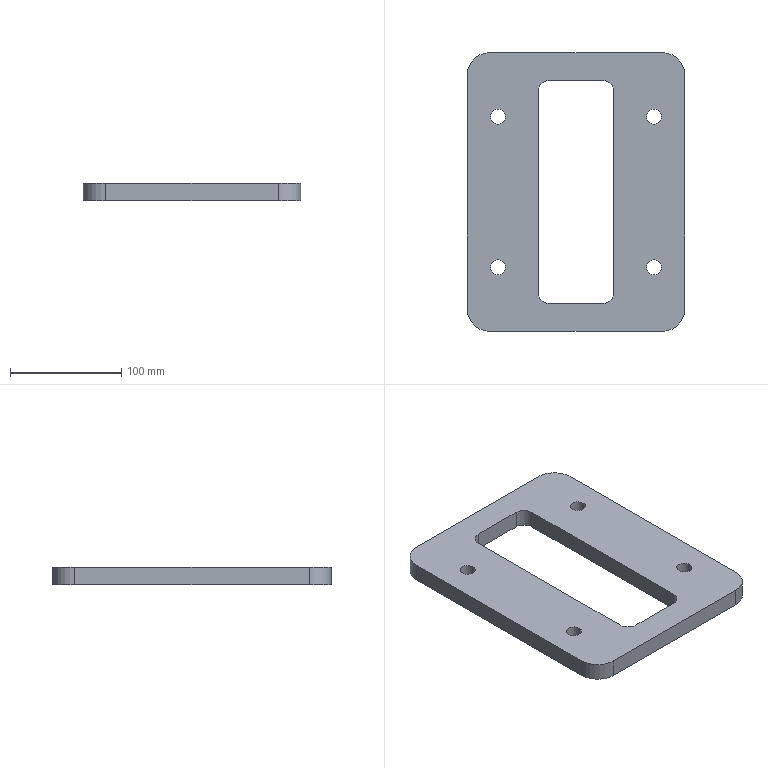Part | SolidWorks | features Fillet 2, Chamfer 1, Extrusion 1, HoleWzd 1 | 1 solid | 26 faces | box 195 x 250 x 16 mm | volume 549119 mm3 | cylinder 16 | plane 10 | commonest cylinder face diameters 13.5 x8 20 x4 40 x4
STEP:
#1=CARTESIAN_POINT('',(-76.75,67.5,-8.));
#2=VERTEX_POINT('',#1);
#3=CARTESIAN_POINT('',(-63.25,67.5,-8.));
#4=VERTEX_POINT('',#3);
#5=CARTESIAN_POINT('',(-70.,67.5,-8.));
#6=DIRECTION('',(0.,0.,1.));
#7=DIRECTION('',(1.,0.,0.));
#8=AXIS2_PLACEMENT_3D('',#5,#6,#7);
#9=CIRCLE('',#8,6.75);
#10=EDGE_CURVE('',#2,#4,#9,.T.);
#11=ORIENTED_EDGE('',*,*,#10,.F.);
#12=CARTESIAN_POINT('',(-76.75,67.5,8.));
#13=VERTEX_POINT('',#12);
#14=CARTESIAN_POINT('',(-76.75,67.5,8.));
#15=DIRECTION('',(0.,0.,1.));
#16=VECTOR('',#15,1000.);
#17=LINE('',#14,#16);
#18=EDGE_CURVE('',#2,#13,#17,.T.);
#19=ORIENTED_EDGE('',*,*,#18,.T.);
#20=CARTESIAN_POINT('',(-63.25,67.5,8.));
#21=VERTEX_POINT('',#20);
#22=CARTESIAN_POINT('',(-70.,67.5,8.));
#23=DIRECTION('',(0.,0.,1.));
#24=DIRECTION('',(1.,0.,0.));
#25=AXIS2_PLACEMENT_3D('',#22,#23,#24);
#26=CIRCLE('',#25,6.75);
#27=EDGE_CURVE('',#13,#21,#26,.T.);
#28=ORIENTED_EDGE('',*,*,#27,.T.);
#29=CARTESIAN_POINT('',(-63.25,67.5,8.));
#30=DIRECTION('',(0.,0.,1.));
#31=VECTOR('',#30,1000.);
#32=LINE('',#29,#31);
#33=EDGE_CURVE('',#4,#21,#32,.T.);
#34=ORIENTED_EDGE('',*,*,#33,.F.);
#35=EDGE_LOOP('',(#11,#19,#28,#34));
#36=FACE_OUTER_BOUND('',#35,.T.);
#37=CARTESIAN_POINT('',(-70.,67.5,8.));
#38=DIRECTION('',(0.,0.,1.));
#39=DIRECTION('',(1.,0.,0.));
#40=AXIS2_PLACEMENT_3D('',#37,#38,#39);
#41=CYLINDRICAL_SURFACE('',#40,6.75);
#42=ADVANCED_FACE('',(#36),#41,.F.);
#43=CARTESIAN_POINT('',(63.25,67.5,-8.));
#44=VERTEX_POINT('',#43);
#45=CARTESIAN_POINT('',(76.75,67.5,-8.));
#46=VERTEX_POINT('',#45);
#47=CARTESIAN_POINT('',(70.,67.5,-8.));
#48=DIRECTION('',(0.,0.,1.));
#49=DIRECTION('',(1.,0.,0.));
#50=AXIS2_PLACEMENT_3D('',#47,#48,#49);
#51=CIRCLE('',#50,6.75);
#52=EDGE_CURVE('',#44,#46,#51,.T.);
#53=ORIENTED_EDGE('',*,*,#52,.F.);
#54=CARTESIAN_POINT('',(63.25,67.5,8.));
#55=VERTEX_POINT('',#54);
#56=CARTESIAN_POINT('',(63.25,67.5,8.));
#57=DIRECTION('',(0.,0.,1.));
#58=VECTOR('',#57,1000.);
#59=LINE('',#56,#58);
#60=EDGE_CURVE('',#44,#55,#59,.T.);
#61=ORIENTED_EDGE('',*,*,#60,.T.);
#62=CARTESIAN_POINT('',(76.75,67.5,8.));
#63=VERTEX_POINT('',#62);
#64=CARTESIAN_POINT('',(70.,67.5,8.));
#65=DIRECTION('',(0.,0.,1.));
#66=DIRECTION('',(1.,0.,0.));
#67=AXIS2_PLACEMENT_3D('',#64,#65,#66);
#68=CIRCLE('',#67,6.75);
#69=EDGE_CURVE('',#55,#63,#68,.T.);
#70=ORIENTED_EDGE('',*,*,#69,.T.);
#71=CARTESIAN_POINT('',(76.75,67.5,8.));
#72=DIRECTION('',(0.,0.,1.));
#73=VECTOR('',#72,1000.);
#74=LINE('',#71,#73);
#75=EDGE_CURVE('',#46,#63,#74,.T.);
#76=ORIENTED_EDGE('',*,*,#75,.F.);
#77=EDGE_LOOP('',(#53,#61,#70,#76));
#78=FACE_OUTER_BOUND('',#77,.T.);
#79=CARTESIAN_POINT('',(70.,67.5,8.));
#80=DIRECTION('',(0.,0.,1.));
#81=DIRECTION('',(1.,0.,0.));
#82=AXIS2_PLACEMENT_3D('',#79,#80,#81);
#83=CYLINDRICAL_SURFACE('',#82,6.75);
#84=ADVANCED_FACE('',(#78),#83,.F.);
#85=CARTESIAN_POINT('',(63.25,-67.5,-8.));
#86=VERTEX_POINT('',#85);
#87=CARTESIAN_POINT('',(76.75,-67.5,-8.));
#88=VERTEX_POINT('',#87);
#89=CARTESIAN_POINT('',(70.,-67.5,-8.));
#90=DIRECTION('',(0.,0.,1.));
#91=DIRECTION('',(1.,0.,0.));
#92=AXIS2_PLACEMENT_3D('',#89,#90,#91);
#93=CIRCLE('',#92,6.75);
#94=EDGE_CURVE('',#86,#88,#93,.T.);
#95=ORIENTED_EDGE('',*,*,#94,.F.);
#96=CARTESIAN_POINT('',(63.25,-67.5,8.));
#97=VERTEX_POINT('',#96);
#98=CARTESIAN_POINT('',(63.25,-67.5,8.));
#99=DIRECTION('',(0.,0.,1.));
#100=VECTOR('',#99,1000.);
#101=LINE('',#98,#100);
#102=EDGE_CURVE('',#86,#97,#101,.T.);
#103=ORIENTED_EDGE('',*,*,#102,.T.);
#104=CARTESIAN_POINT('',(76.75,-67.5,8.));
#105=VERTEX_POINT('',#104);
#106=CARTESIAN_POINT('',(70.,-67.5,8.));
#107=DIRECTION('',(0.,0.,1.));
#108=DIRECTION('',(1.,0.,0.));
#109=AXIS2_PLACEMENT_3D('',#106,#107,#108);
#110=CIRCLE('',#109,6.75);
#111=EDGE_CURVE('',#97,#105,#110,.T.);
#112=ORIENTED_EDGE('',*,*,#111,.T.);
#113=CARTESIAN_POINT('',(76.75,-67.5,8.));
#114=DIRECTION('',(0.,0.,1.));
#115=VECTOR('',#114,1000.);
#116=LINE('',#113,#115);
#117=EDGE_CURVE('',#88,#105,#116,.T.);
#118=ORIENTED_EDGE('',*,*,#117,.F.);
#119=EDGE_LOOP('',(#95,#103,#112,#118));
#120=FACE_OUTER_BOUND('',#119,.T.);
#121=CARTESIAN_POINT('',(70.,-67.5,8.));
#122=DIRECTION('',(0.,0.,1.));
#123=DIRECTION('',(1.,0.,0.));
#124=AXIS2_PLACEMENT_3D('',#121,#122,#123);
#125=CYLINDRICAL_SURFACE('',#124,6.75);
#126=ADVANCED_FACE('',(#120),#125,.F.);
#127=CARTESIAN_POINT('',(-76.75,-67.5,-8.));
#128=VERTEX_POINT('',#127);
#129=CARTESIAN_POINT('',(-63.25,-67.5,-8.));
#130=VERTEX_POINT('',#129);
#131=CARTESIAN_POINT('',(-70.,-67.5,-8.));
#132=DIRECTION('',(0.,0.,1.));
#133=DIRECTION('',(1.,0.,0.));
#134=AXIS2_PLACEMENT_3D('',#131,#132,#133);
#135=CIRCLE('',#134,6.75);
#136=EDGE_CURVE('',#128,#130,#135,.T.);
#137=ORIENTED_EDGE('',*,*,#136,.F.);
#138=CARTESIAN_POINT('',(-76.75,-67.5,8.));
#139=VERTEX_POINT('',#138);
#140=CARTESIAN_POINT('',(-76.75,-67.5,8.));
#141=DIRECTION('',(0.,0.,1.));
#142=VECTOR('',#141,1000.);
#143=LINE('',#140,#142);
#144=EDGE_CURVE('',#128,#139,#143,.T.);
#145=ORIENTED_EDGE('',*,*,#144,.T.);
#146=CARTESIAN_POINT('',(-63.25,-67.5,8.));
#147=VERTEX_POINT('',#146);
#148=CARTESIAN_POINT('',(-70.,-67.5,8.));
#149=DIRECTION('',(0.,0.,1.));
#150=DIRECTION('',(1.,0.,0.));
#151=AXIS2_PLACEMENT_3D('',#148,#149,#150);
#152=CIRCLE('',#151,6.75);
#153=EDGE_CURVE('',#139,#147,#152,.T.);
#154=ORIENTED_EDGE('',*,*,#153,.T.);
#155=CARTESIAN_POINT('',(-63.25,-67.5,8.));
#156=DIRECTION('',(0.,0.,1.));
#157=VECTOR('',#156,1000.);
#158=LINE('',#155,#157);
#159=EDGE_CURVE('',#130,#147,#158,.T.);
#160=ORIENTED_EDGE('',*,*,#159,.F.);
#161=EDGE_LOOP('',(#137,#145,#154,#160));
#162=FACE_OUTER_BOUND('',#161,.T.);
#163=CARTESIAN_POINT('',(-70.,-67.5,8.));
#164=DIRECTION('',(0.,0.,1.));
#165=DIRECTION('',(1.,0.,0.));
#166=AXIS2_PLACEMENT_3D('',#163,#164,#165);
#167=CYLINDRICAL_SURFACE('',#166,6.75);
#168=ADVANCED_FACE('',(#162),#167,.F.);
#169=CARTESIAN_POINT('',(-70.,67.5,8.));
#170=DIRECTION('',(0.,0.,1.));
#171=DIRECTION('',(1.,0.,0.));
#172=AXIS2_PLACEMENT_3D('',#169,#170,#171);
#173=CIRCLE('',#172,6.75);
#174=EDGE_CURVE('',#21,#13,#173,.T.);
#175=ORIENTED_EDGE('',*,*,#174,.F.);
#176=ORIENTED_EDGE('',*,*,#27,.F.);
#177=EDGE_LOOP('',(#175,#176));
#178=FACE_BOUND('',#177,.T.);
#179=CARTESIAN_POINT('',(70.,67.5,8.));
#180=DIRECTION('',(0.,0.,1.));
#181=DIRECTION('',(1.,0.,0.));
#182=AXIS2_PLACEMENT_3D('',#179,#180,#181);
#183=CIRCLE('',#182,6.75);
#184=EDGE_CURVE('',#63,#55,#183,.T.);
#185=ORIENTED_EDGE('',*,*,#184,.F.);
#186=ORIENTED_EDGE('',*,*,#69,.F.);
#187=EDGE_LOOP('',(#185,#186));
#188=FACE_BOUND('',#187,.T.);
#189=CARTESIAN_POINT('',(70.,-67.5,8.));
#190=DIRECTION('',(0.,0.,1.));
#191=DIRECTION('',(1.,0.,0.));
#192=AXIS2_PLACEMENT_3D('',#189,#190,#191);
#193=CIRCLE('',#192,6.75);
#194=EDGE_CURVE('',#105,#97,#193,.T.);
#195=ORIENTED_EDGE('',*,*,#194,.F.);
#196=ORIENTED_EDGE('',*,*,#111,.F.);
#197=EDGE_LOOP('',(#195,#196));
#198=FACE_BOUND('',#197,.T.);
#199=CARTESIAN_POINT('',(-70.,-67.5,8.));
#200=DIRECTION('',(0.,0.,1.));
#201=DIRECTION('',(1.,0.,0.));
#202=AXIS2_PLACEMENT_3D('',#199,#200,#201);
#203=CIRCLE('',#202,6.75);
#204=EDGE_CURVE('',#147,#139,#203,.T.);
#205=ORIENTED_EDGE('',*,*,#204,.F.);
#206=ORIENTED_EDGE('',*,*,#153,.F.);
#207=EDGE_LOOP('',(#205,#206));
#208=FACE_BOUND('',#207,.T.);
#209=CARTESIAN_POINT('',(97.5,-105.,8.));
#210=VERTEX_POINT('',#209);
#211=CARTESIAN_POINT('',(97.5,105.,8.));
#212=VERTEX_POINT('',#211);
#213=CARTESIAN_POINT('',(97.5,-125.,8.));
#214=DIRECTION('',(0.,1.,0.));
#215=VECTOR('',#214,1000.);
#216=LINE('',#213,#215);
#217=EDGE_CURVE('',#210,#212,#216,.T.);
#218=ORIENTED_EDGE('',*,*,#217,.T.);
#219=CARTESIAN_POINT('',(77.5,125.,8.));
#220=VERTEX_POINT('',#219);
#221=CARTESIAN_POINT('',(77.5,105.,8.));
#222=DIRECTION('',(0.,0.,1.));
#223=DIRECTION('',(1.,0.,0.));
#224=AXIS2_PLACEMENT_3D('',#221,#222,#223);
#225=CIRCLE('',#224,20.);
#226=EDGE_CURVE('',#212,#220,#225,.T.);
#227=ORIENTED_EDGE('',*,*,#226,.T.);
#228=CARTESIAN_POINT('',(-77.5,125.,8.));
#229=VERTEX_POINT('',#228);
#230=CARTESIAN_POINT('',(97.5,125.,8.));
#231=DIRECTION('',(-1.,0.,0.));
#232=VECTOR('',#231,1000.);
#233=LINE('',#230,#232);
#234=EDGE_CURVE('',#220,#229,#233,.T.);
#235=ORIENTED_EDGE('',*,*,#234,.T.);
#236=CARTESIAN_POINT('',(-97.5,105.,8.));
#237=VERTEX_POINT('',#236);
#238=CARTESIAN_POINT('',(-77.5,105.,8.));
#239=DIRECTION('',(0.,0.,1.));
#240=DIRECTION('',(1.,0.,0.));
#241=AXIS2_PLACEMENT_3D('',#238,#239,#240);
#242=CIRCLE('',#241,20.);
#243=EDGE_CURVE('',#229,#237,#242,.T.);
#244=ORIENTED_EDGE('',*,*,#243,.T.);
#245=CARTESIAN_POINT('',(-97.5,-105.,8.));
#246=VERTEX_POINT('',#245);
#247=CARTESIAN_POINT('',(-97.5,-125.,8.));
#248=DIRECTION('',(0.,-1.,0.));
#249=VECTOR('',#248,1000.);
#250=LINE('',#247,#249);
#251=EDGE_CURVE('',#237,#246,#250,.T.);
#252=ORIENTED_EDGE('',*,*,#251,.T.);
#253=CARTESIAN_POINT('',(-77.5,-125.,8.));
#254=VERTEX_POINT('',#253);
#255=CARTESIAN_POINT('',(-77.5,-105.,8.));
#256=DIRECTION('',(0.,0.,1.));
#257=DIRECTION('',(1.,0.,0.));
#258=AXIS2_PLACEMENT_3D('',#255,#256,#257);
#259=CIRCLE('',#258,20.);
#260=EDGE_CURVE('',#246,#254,#259,.T.);
#261=ORIENTED_EDGE('',*,*,#260,.T.);
#262=CARTESIAN_POINT('',(77.5,-125.,8.));
#263=VERTEX_POINT('',#262);
#264=CARTESIAN_POINT('',(97.5,-125.,8.));
#265=DIRECTION('',(1.,0.,0.));
#266=VECTOR('',#265,1000.);
#267=LINE('',#264,#266);
#268=EDGE_CURVE('',#254,#263,#267,.T.);
#269=ORIENTED_EDGE('',*,*,#268,.T.);
#270=CARTESIAN_POINT('',(77.5,-105.,8.));
#271=DIRECTION('',(0.,0.,1.));
#272=DIRECTION('',(1.,0.,0.));
#273=AXIS2_PLACEMENT_3D('',#270,#271,#272);
#274=CIRCLE('',#273,20.);
#275=EDGE_CURVE('',#263,#210,#274,.T.);
#276=ORIENTED_EDGE('',*,*,#275,.T.);
#277=EDGE_LOOP('',(#218,#227,#235,#244,#252,#261,#269,#276));
#278=FACE_OUTER_BOUND('',#277,.T.);
#279=CARTESIAN_POINT('',(-24.,-100.,8.));
#280=VERTEX_POINT('',#279);
#281=CARTESIAN_POINT('',(24.,-100.,8.));
#282=VERTEX_POINT('',#281);
#283=CARTESIAN_POINT('',(34.,-100.,8.));
#284=DIRECTION('',(1.,0.,0.));
#285=VECTOR('',#284,1000.);
#286=LINE('',#283,#285);
#287=EDGE_CURVE('',#280,#282,#286,.T.);
#288=ORIENTED_EDGE('',*,*,#287,.F.);
#289=CARTESIAN_POINT('',(-34.,-90.,8.));
#290=VERTEX_POINT('',#289);
#291=CARTESIAN_POINT('',(-24.,-90.,8.));
#292=DIRECTION('',(0.,0.,-1.));
#293=DIRECTION('',(1.,0.,0.));
#294=AXIS2_PLACEMENT_3D('',#291,#292,#293);
#295=CIRCLE('',#294,10.);
#296=EDGE_CURVE('',#280,#290,#295,.T.);
#297=ORIENTED_EDGE('',*,*,#296,.T.);
#298=CARTESIAN_POINT('',(-34.,90.,8.));
#299=VERTEX_POINT('',#298);
#300=CARTESIAN_POINT('',(-34.,-100.,8.));
#301=DIRECTION('',(0.,-1.,0.));
#302=VECTOR('',#301,1000.);
#303=LINE('',#300,#302);
#304=EDGE_CURVE('',#299,#290,#303,.T.);
#305=ORIENTED_EDGE('',*,*,#304,.F.);
#306=CARTESIAN_POINT('',(-24.,100.,8.));
#307=VERTEX_POINT('',#306);
#308=CARTESIAN_POINT('',(-24.,90.,8.));
#309=DIRECTION('',(0.,0.,-1.));
#310=DIRECTION('',(1.,0.,0.));
#311=AXIS2_PLACEMENT_3D('',#308,#309,#310);
#312=CIRCLE('',#311,10.);
#313=EDGE_CURVE('',#299,#307,#312,.T.);
#314=ORIENTED_EDGE('',*,*,#313,.T.);
#315=CARTESIAN_POINT('',(24.,100.,8.));
#316=VERTEX_POINT('',#315);
#317=CARTESIAN_POINT('',(34.,100.,8.));
#318=DIRECTION('',(-1.,0.,0.));
#319=VECTOR('',#318,1000.);
#320=LINE('',#317,#319);
#321=EDGE_CURVE('',#316,#307,#320,.T.);
#322=ORIENTED_EDGE('',*,*,#321,.F.);
#323=CARTESIAN_POINT('',(34.,90.,8.));
#324=VERTEX_POINT('',#323);
#325=CARTESIAN_POINT('',(24.,90.,8.));
#326=DIRECTION('',(0.,0.,-1.));
#327=DIRECTION('',(1.,0.,0.));
#328=AXIS2_PLACEMENT_3D('',#325,#326,#327);
#329=CIRCLE('',#328,10.);
#330=EDGE_CURVE('',#316,#324,#329,.T.);
#331=ORIENTED_EDGE('',*,*,#330,.T.);
#332=CARTESIAN_POINT('',(34.,-90.,8.));
#333=VERTEX_POINT('',#332);
#334=CARTESIAN_POINT('',(34.,-100.,8.));
#335=DIRECTION('',(0.,1.,0.));
#336=VECTOR('',#335,1000.);
#337=LINE('',#334,#336);
#338=EDGE_CURVE('',#333,#324,#337,.T.);
#339=ORIENTED_EDGE('',*,*,#338,.F.);
#340=CARTESIAN_POINT('',(24.,-90.,8.));
#341=DIRECTION('',(0.,0.,-1.));
#342=DIRECTION('',(1.,0.,0.));
#343=AXIS2_PLACEMENT_3D('',#340,#341,#342);
#344=CIRCLE('',#343,10.);
#345=EDGE_CURVE('',#333,#282,#344,.T.);
#346=ORIENTED_EDGE('',*,*,#345,.T.);
#347=EDGE_LOOP('',(#288,#297,#305,#314,#322,#331,#339,#346));
#348=FACE_BOUND('',#347,.T.);
#349=CARTESIAN_POINT('',(0.,0.,8.));
#350=DIRECTION('',(0.,0.,1.));
#351=DIRECTION('',(1.,0.,0.));
#352=AXIS2_PLACEMENT_3D('',#349,#350,#351);
#353=PLANE('',#352);
#354=ADVANCED_FACE('',(#178,#188,#198,#208,#278,#348),#353,.T.);
#355=CARTESIAN_POINT('',(-70.,67.5,-8.));
#356=DIRECTION('',(0.,0.,1.));
#357=DIRECTION('',(1.,0.,0.));
#358=AXIS2_PLACEMENT_3D('',#355,#356,#357);
#359=CIRCLE('',#358,6.75);
#360=EDGE_CURVE('',#4,#2,#359,.T.);
#361=ORIENTED_EDGE('',*,*,#360,.T.);
#362=ORIENTED_EDGE('',*,*,#10,.T.);
#363=EDGE_LOOP('',(#361,#362));
#364=FACE_BOUND('',#363,.T.);
#365=CARTESIAN_POINT('',(70.,67.5,-8.));
#366=DIRECTION('',(0.,0.,1.));
#367=DIRECTION('',(1.,0.,0.));
#368=AXIS2_PLACEMENT_3D('',#365,#366,#367);
#369=CIRCLE('',#368,6.75);
#370=EDGE_CURVE('',#46,#44,#369,.T.);
#371=ORIENTED_EDGE('',*,*,#370,.T.);
#372=ORIENTED_EDGE('',*,*,#52,.T.);
#373=EDGE_LOOP('',(#371,#372));
#374=FACE_BOUND('',#373,.T.);
#375=CARTESIAN_POINT('',(70.,-67.5,-8.));
#376=DIRECTION('',(0.,0.,1.));
#377=DIRECTION('',(1.,0.,0.));
#378=AXIS2_PLACEMENT_3D('',#375,#376,#377);
#379=CIRCLE('',#378,6.75);
#380=EDGE_CURVE('',#88,#86,#379,.T.);
#381=ORIENTED_EDGE('',*,*,#380,.T.);
#382=ORIENTED_EDGE('',*,*,#94,.T.);
#383=EDGE_LOOP('',(#381,#382));
#384=FACE_BOUND('',#383,.T.);
#385=CARTESIAN_POINT('',(-70.,-67.5,-8.));
#386=DIRECTION('',(0.,0.,1.));
#387=DIRECTION('',(1.,0.,0.));
#388=AXIS2_PLACEMENT_3D('',#385,#386,#387);
#389=CIRCLE('',#388,6.75);
#390=EDGE_CURVE('',#130,#128,#389,.T.);
#391=ORIENTED_EDGE('',*,*,#390,.T.);
#392=ORIENTED_EDGE('',*,*,#136,.T.);
#393=EDGE_LOOP('',(#391,#392));
#394=FACE_BOUND('',#393,.T.);
#395=CARTESIAN_POINT('',(77.5,125.,-8.));
#396=VERTEX_POINT('',#395);
#397=CARTESIAN_POINT('',(-77.5,125.,-8.));
#398=VERTEX_POINT('',#397);
#399=CARTESIAN_POINT('',(97.5,125.,-8.));
#400=DIRECTION('',(-1.,0.,0.));
#401=VECTOR('',#400,1000.);
#402=LINE('',#399,#401);
#403=EDGE_CURVE('',#396,#398,#402,.T.);
#404=ORIENTED_EDGE('',*,*,#403,.F.);
#405=CARTESIAN_POINT('',(97.5,105.,-8.));
#406=VERTEX_POINT('',#405);
#407=CARTESIAN_POINT('',(77.5,105.,-8.));
#408=DIRECTION('',(0.,0.,-1.));
#409=DIRECTION('',(1.,0.,0.));
#410=AXIS2_PLACEMENT_3D('',#407,#408,#409);
#411=CIRCLE('',#410,20.);
#412=EDGE_CURVE('',#396,#406,#411,.T.);
#413=ORIENTED_EDGE('',*,*,#412,.T.);
#414=CARTESIAN_POINT('',(97.5,-105.,-8.));
#415=VERTEX_POINT('',#414);
#416=CARTESIAN_POINT('',(97.5,-125.,-8.));
#417=DIRECTION('',(0.,1.,0.));
#418=VECTOR('',#417,1000.);
#419=LINE('',#416,#418);
#420=EDGE_CURVE('',#415,#406,#419,.T.);
#421=ORIENTED_EDGE('',*,*,#420,.F.);
#422=CARTESIAN_POINT('',(77.5,-125.,-8.));
#423=VERTEX_POINT('',#422);
#424=CARTESIAN_POINT('',(77.5,-105.,-8.));
#425=DIRECTION('',(0.,0.,-1.));
#426=DIRECTION('',(1.,0.,0.));
#427=AXIS2_PLACEMENT_3D('',#424,#425,#426);
#428=CIRCLE('',#427,20.);
#429=EDGE_CURVE('',#415,#423,#428,.T.);
#430=ORIENTED_EDGE('',*,*,#429,.T.);
#431=CARTESIAN_POINT('',(-77.5,-125.,-8.));
#432=VERTEX_POINT('',#431);
#433=CARTESIAN_POINT('',(97.5,-125.,-8.));
#434=DIRECTION('',(1.,0.,0.));
#435=VECTOR('',#434,1000.);
#436=LINE('',#433,#435);
#437=EDGE_CURVE('',#432,#423,#436,.T.);
#438=ORIENTED_EDGE('',*,*,#437,.F.);
#439=CARTESIAN_POINT('',(-97.5,-105.,-8.));
#440=VERTEX_POINT('',#439);
#441=CARTESIAN_POINT('',(-77.5,-105.,-8.));
#442=DIRECTION('',(0.,0.,-1.));
#443=DIRECTION('',(1.,0.,0.));
#444=AXIS2_PLACEMENT_3D('',#441,#442,#443);
#445=CIRCLE('',#444,20.);
#446=EDGE_CURVE('',#432,#440,#445,.T.);
#447=ORIENTED_EDGE('',*,*,#446,.T.);
#448=CARTESIAN_POINT('',(-97.5,105.,-8.));
#449=VERTEX_POINT('',#448);
#450=CARTESIAN_POINT('',(-97.5,-125.,-8.));
#451=DIRECTION('',(0.,-1.,0.));
#452=VECTOR('',#451,1000.);
#453=LINE('',#450,#452);
#454=EDGE_CURVE('',#449,#440,#453,.T.);
#455=ORIENTED_EDGE('',*,*,#454,.F.);
#456=CARTESIAN_POINT('',(-77.5,105.,-8.));
#457=DIRECTION('',(0.,0.,-1.));
#458=DIRECTION('',(1.,0.,0.));
#459=AXIS2_PLACEMENT_3D('',#456,#457,#458);
#460=CIRCLE('',#459,20.);
#461=EDGE_CURVE('',#449,#398,#460,.T.);
#462=ORIENTED_EDGE('',*,*,#461,.T.);
#463=EDGE_LOOP('',(#404,#413,#421,#430,#438,#447,#455,#462));
#464=FACE_OUTER_BOUND('',#463,.T.);
#465=CARTESIAN_POINT('',(24.,100.,-8.));
#466=VERTEX_POINT('',#465);
#467=CARTESIAN_POINT('',(-24.,100.,-8.));
#468=VERTEX_POINT('',#467);
#469=CARTESIAN_POINT('',(34.,100.,-8.));
#470=DIRECTION('',(-1.,0.,0.));
#471=VECTOR('',#470,1000.);
#472=LINE('',#469,#471);
#473=EDGE_CURVE('',#466,#468,#472,.T.);
#474=ORIENTED_EDGE('',*,*,#473,.T.);
#475=CARTESIAN_POINT('',(-34.,90.,-8.));
#476=VERTEX_POINT('',#475);
#477=CARTESIAN_POINT('',(-24.,90.,-8.));
#478=DIRECTION('',(0.,0.,1.));
#479=DIRECTION('',(1.,0.,0.));
#480=AXIS2_PLACEMENT_3D('',#477,#478,#479);
#481=CIRCLE('',#480,10.);
#482=EDGE_CURVE('',#468,#476,#481,.T.);
#483=ORIENTED_EDGE('',*,*,#482,.T.);
#484=CARTESIAN_POINT('',(-34.,-90.,-8.));
#485=VERTEX_POINT('',#484);
#486=CARTESIAN_POINT('',(-34.,-100.,-8.));
#487=DIRECTION('',(0.,-1.,0.));
#488=VECTOR('',#487,1000.);
#489=LINE('',#486,#488);
#490=EDGE_CURVE('',#476,#485,#489,.T.);
#491=ORIENTED_EDGE('',*,*,#490,.T.);
#492=CARTESIAN_POINT('',(-24.,-100.,-8.));
#493=VERTEX_POINT('',#492);
#494=CARTESIAN_POINT('',(-24.,-90.,-8.));
#495=DIRECTION('',(0.,0.,1.));
#496=DIRECTION('',(1.,0.,0.));
#497=AXIS2_PLACEMENT_3D('',#494,#495,#496);
#498=CIRCLE('',#497,10.);
#499=EDGE_CURVE('',#485,#493,#498,.T.);
#500=ORIENTED_EDGE('',*,*,#499,.T.);
#501=CARTESIAN_POINT('',(24.,-100.,-8.));
#502=VERTEX_POINT('',#501);
#503=CARTESIAN_POINT('',(34.,-100.,-8.));
#504=DIRECTION('',(1.,0.,0.));
#505=VECTOR('',#504,1000.);
#506=LINE('',#503,#505);
#507=EDGE_CURVE('',#493,#502,#506,.T.);
#508=ORIENTED_EDGE('',*,*,#507,.T.);
#509=CARTESIAN_POINT('',(34.,-90.,-8.));
#510=VERTEX_POINT('',#509);
#511=CARTESIAN_POINT('',(24.,-90.,-8.));
#512=DIRECTION('',(0.,0.,1.));
#513=DIRECTION('',(1.,0.,0.));
#514=AXIS2_PLACEMENT_3D('',#511,#512,#513);
#515=CIRCLE('',#514,10.);
#516=EDGE_CURVE('',#502,#510,#515,.T.);
#517=ORIENTED_EDGE('',*,*,#516,.T.);
#518=CARTESIAN_POINT('',(34.,90.,-8.));
#519=VERTEX_POINT('',#518);
#520=CARTESIAN_POINT('',(34.,-100.,-8.));
#521=DIRECTION('',(0.,1.,0.));
#522=VECTOR('',#521,1000.);
#523=LINE('',#520,#522);
#524=EDGE_CURVE('',#510,#519,#523,.T.);
#525=ORIENTED_EDGE('',*,*,#524,.T.);
#526=CARTESIAN_POINT('',(24.,90.,-8.));
#527=DIRECTION('',(0.,0.,1.));
#528=DIRECTION('',(1.,0.,0.));
#529=AXIS2_PLACEMENT_3D('',#526,#527,#528);
#530=CIRCLE('',#529,10.);
#531=EDGE_CURVE('',#519,#466,#530,.T.);
#532=ORIENTED_EDGE('',*,*,#531,.T.);
#533=EDGE_LOOP('',(#474,#483,#491,#500,#508,#517,#525,#532));
#534=FACE_BOUND('',#533,.T.);
#535=CARTESIAN_POINT('',(0.,0.,-8.));
#536=DIRECTION('',(0.,0.,1.));
#537=DIRECTION('',(1.,0.,0.));
#538=AXIS2_PLACEMENT_3D('',#535,#536,#537);
#539=PLANE('',#538);
#540=ADVANCED_FACE('',(#364,#374,#384,#394,#464,#534),#539,.F.);
#541=ORIENTED_EDGE('',*,*,#454,.T.);
#542=CARTESIAN_POINT('',(-97.5,-105.,8.));
#543=DIRECTION('',(0.,0.,1.));
#544=VECTOR('',#543,1000.);
#545=LINE('',#542,#544);
#546=EDGE_CURVE('',#440,#246,#545,.T.);
#547=ORIENTED_EDGE('',*,*,#546,.T.);
#548=ORIENTED_EDGE('',*,*,#251,.F.);
#549=CARTESIAN_POINT('',(-97.5,105.,8.));
#550=DIRECTION('',(0.,0.,-1.));
#551=VECTOR('',#550,1000.);
#552=LINE('',#549,#551);
#553=EDGE_CURVE('',#237,#449,#552,.T.);
#554=ORIENTED_EDGE('',*,*,#553,.T.);
#555=EDGE_LOOP('',(#541,#547,#548,#554));
#556=FACE_OUTER_BOUND('',#555,.T.);
#557=CARTESIAN_POINT('',(-97.5,-125.,8.));
#558=DIRECTION('',(1.,0.,0.));
#559=DIRECTION('',(0.,0.,-1.));
#560=AXIS2_PLACEMENT_3D('',#557,#558,#559);
#561=PLANE('',#560);
#562=ADVANCED_FACE('',(#556),#561,.F.);
#563=ORIENTED_EDGE('',*,*,#437,.T.);
#564=CARTESIAN_POINT('',(77.5,-125.,8.));
#565=DIRECTION('',(0.,0.,1.));
#566=VECTOR('',#565,1000.);
#567=LINE('',#564,#566);
#568=EDGE_CURVE('',#423,#263,#567,.T.);
#569=ORIENTED_EDGE('',*,*,#568,.T.);
#570=ORIENTED_EDGE('',*,*,#268,.F.);
#571=CARTESIAN_POINT('',(-77.5,-125.,8.));
#572=DIRECTION('',(0.,0.,-1.));
#573=VECTOR('',#572,1000.);
#574=LINE('',#571,#573);
#575=EDGE_CURVE('',#254,#432,#574,.T.);
#576=ORIENTED_EDGE('',*,*,#575,.T.);
#577=EDGE_LOOP('',(#563,#569,#570,#576));
#578=FACE_OUTER_BOUND('',#577,.T.);
#579=CARTESIAN_POINT('',(97.5,-125.,8.));
#580=DIRECTION('',(0.,1.,0.));
#581=DIRECTION('',(-1.,0.,0.));
#582=AXIS2_PLACEMENT_3D('',#579,#580,#581);
#583=PLANE('',#582);
#584=ADVANCED_FACE('',(#578),#583,.F.);
#585=ORIENTED_EDGE('',*,*,#420,.T.);
#586=CARTESIAN_POINT('',(97.5,105.,8.));
#587=DIRECTION('',(0.,0.,1.));
#588=VECTOR('',#587,1000.);
#589=LINE('',#586,#588);
#590=EDGE_CURVE('',#406,#212,#589,.T.);
#591=ORIENTED_EDGE('',*,*,#590,.T.);
#592=ORIENTED_EDGE('',*,*,#217,.F.);
#593=CARTESIAN_POINT('',(97.5,-105.,8.));
#594=DIRECTION('',(0.,0.,-1.));
#595=VECTOR('',#594,1000.);
#596=LINE('',#593,#595);
#597=EDGE_CURVE('',#210,#415,#596,.T.);
#598=ORIENTED_EDGE('',*,*,#597,.T.);
#599=EDGE_LOOP('',(#585,#591,#592,#598));
#600=FACE_OUTER_BOUND('',#599,.T.);
#601=CARTESIAN_POINT('',(97.5,-125.,8.));
#602=DIRECTION('',(-1.,0.,0.));
#603=DIRECTION('',(0.,0.,1.));
#604=AXIS2_PLACEMENT_3D('',#601,#602,#603);
#605=PLANE('',#604);
#606=ADVANCED_FACE('',(#600),#605,.F.);
#607=ORIENTED_EDGE('',*,*,#234,.F.);
#608=CARTESIAN_POINT('',(77.5,125.,8.));
#609=DIRECTION('',(0.,0.,-1.));
#610=VECTOR('',#609,1000.);
#611=LINE('',#608,#610);
#612=EDGE_CURVE('',#220,#396,#611,.T.);
#613=ORIENTED_EDGE('',*,*,#612,.T.);
#614=ORIENTED_EDGE('',*,*,#403,.T.);
#615=CARTESIAN_POINT('',(-77.5,125.,8.));
#616=DIRECTION('',(0.,0.,1.));
#617=VECTOR('',#616,1000.);
#618=LINE('',#615,#617);
#619=EDGE_CURVE('',#398,#229,#618,.T.);
#620=ORIENTED_EDGE('',*,*,#619,.T.);
#621=EDGE_LOOP('',(#607,#613,#614,#620));
#622=FACE_OUTER_BOUND('',#621,.T.);
#623=CARTESIAN_POINT('',(97.5,125.,8.));
#624=DIRECTION('',(0.,-1.,0.));
#625=DIRECTION('',(1.,0.,0.));
#626=AXIS2_PLACEMENT_3D('',#623,#624,#625);
#627=PLANE('',#626);
#628=ADVANCED_FACE('',(#622),#627,.F.);
#629=ORIENTED_EDGE('',*,*,#490,.F.);
#630=CARTESIAN_POINT('',(-34.,90.,8.));
#631=DIRECTION('',(0.,0.,1.));
#632=VECTOR('',#631,1000.);
#633=LINE('',#630,#632);
#634=EDGE_CURVE('',#476,#299,#633,.T.);
#635=ORIENTED_EDGE('',*,*,#634,.T.);
#636=ORIENTED_EDGE('',*,*,#304,.T.);
#637=CARTESIAN_POINT('',(-34.,-90.,-8.));
#638=DIRECTION('',(0.,0.,-1.));
#639=VECTOR('',#638,1000.);
#640=LINE('',#637,#639);
#641=EDGE_CURVE('',#290,#485,#640,.T.);
#642=ORIENTED_EDGE('',*,*,#641,.T.);
#643=EDGE_LOOP('',(#629,#635,#636,#642));
#644=FACE_OUTER_BOUND('',#643,.T.);
#645=CARTESIAN_POINT('',(-34.,-100.,8.));
#646=DIRECTION('',(1.,0.,0.));
#647=DIRECTION('',(0.,1.,0.));
#648=AXIS2_PLACEMENT_3D('',#645,#646,#647);
#649=PLANE('',#648);
#650=ADVANCED_FACE('',(#644),#649,.T.);
#651=ORIENTED_EDGE('',*,*,#287,.T.);
#652=CARTESIAN_POINT('',(24.,-100.,-8.));
#653=DIRECTION('',(0.,0.,-1.));
#654=VECTOR('',#653,1000.);
#655=LINE('',#652,#654);
#656=EDGE_CURVE('',#282,#502,#655,.T.);
#657=ORIENTED_EDGE('',*,*,#656,.T.);
#658=ORIENTED_EDGE('',*,*,#507,.F.);
#659=CARTESIAN_POINT('',(-24.,-100.,8.));
#660=DIRECTION('',(0.,0.,1.));
#661=VECTOR('',#660,1000.);
#662=LINE('',#659,#661);
#663=EDGE_CURVE('',#493,#280,#662,.T.);
#664=ORIENTED_EDGE('',*,*,#663,.T.);
#665=EDGE_LOOP('',(#651,#657,#658,#664));
#666=FACE_OUTER_BOUND('',#665,.T.);
#667=CARTESIAN_POINT('',(34.,-100.,8.));
#668=DIRECTION('',(0.,1.,0.));
#669=DIRECTION('',(-1.,0.,0.));
#670=AXIS2_PLACEMENT_3D('',#667,#668,#669);
#671=PLANE('',#670);
#672=ADVANCED_FACE('',(#666),#671,.T.);
#673=ORIENTED_EDGE('',*,*,#338,.T.);
#674=CARTESIAN_POINT('',(34.,90.,-8.));
#675=DIRECTION('',(0.,0.,-1.));
#676=VECTOR('',#675,1000.);
#677=LINE('',#674,#676);
#678=EDGE_CURVE('',#324,#519,#677,.T.);
#679=ORIENTED_EDGE('',*,*,#678,.T.);
#680=ORIENTED_EDGE('',*,*,#524,.F.);
#681=CARTESIAN_POINT('',(34.,-90.,8.));
#682=DIRECTION('',(0.,0.,1.));
#683=VECTOR('',#682,1000.);
#684=LINE('',#681,#683);
#685=EDGE_CURVE('',#510,#333,#684,.T.);
#686=ORIENTED_EDGE('',*,*,#685,.T.);
#687=EDGE_LOOP('',(#673,#679,#680,#686));
#688=FACE_OUTER_BOUND('',#687,.T.);
#689=CARTESIAN_POINT('',(34.,-100.,8.));
#690=DIRECTION('',(-1.,0.,0.));
#691=DIRECTION('',(0.,-1.,0.));
#692=AXIS2_PLACEMENT_3D('',#689,#690,#691);
#693=PLANE('',#692);
#694=ADVANCED_FACE('',(#688),#693,.T.);
#695=ORIENTED_EDGE('',*,*,#473,.F.);
#696=CARTESIAN_POINT('',(24.,100.,8.));
#697=DIRECTION('',(0.,0.,1.));
#698=VECTOR('',#697,1000.);
#699=LINE('',#696,#698);
#700=EDGE_CURVE('',#466,#316,#699,.T.);
#701=ORIENTED_EDGE('',*,*,#700,.T.);
#702=ORIENTED_EDGE('',*,*,#321,.T.);
#703=CARTESIAN_POINT('',(-24.,100.,-8.));
#704=DIRECTION('',(0.,0.,-1.));
#705=VECTOR('',#704,1000.);
#706=LINE('',#703,#705);
#707=EDGE_CURVE('',#307,#468,#706,.T.);
#708=ORIENTED_EDGE('',*,*,#707,.T.);
#709=EDGE_LOOP('',(#695,#701,#702,#708));
#710=FACE_OUTER_BOUND('',#709,.T.);
#711=CARTESIAN_POINT('',(34.,100.,8.));
#712=DIRECTION('',(0.,-1.,0.));
#713=DIRECTION('',(0.,0.,-1.));
#714=AXIS2_PLACEMENT_3D('',#711,#712,#713);
#715=PLANE('',#714);
#716=ADVANCED_FACE('',(#710),#715,.T.);
#717=ORIENTED_EDGE('',*,*,#144,.F.);
#718=ORIENTED_EDGE('',*,*,#390,.F.);
#719=ORIENTED_EDGE('',*,*,#159,.T.);
#720=ORIENTED_EDGE('',*,*,#204,.T.);
#721=EDGE_LOOP('',(#717,#718,#719,#720));
#722=FACE_OUTER_BOUND('',#721,.T.);
#723=CARTESIAN_POINT('',(-70.,-67.5,8.));
#724=DIRECTION('',(0.,0.,1.));
#725=DIRECTION('',(1.,0.,0.));
#726=AXIS2_PLACEMENT_3D('',#723,#724,#725);
#727=CYLINDRICAL_SURFACE('',#726,6.75);
#728=ADVANCED_FACE('',(#722),#727,.F.);
#729=ORIENTED_EDGE('',*,*,#102,.F.);
#730=ORIENTED_EDGE('',*,*,#380,.F.);
#731=ORIENTED_EDGE('',*,*,#117,.T.);
#732=ORIENTED_EDGE('',*,*,#194,.T.);
#733=EDGE_LOOP('',(#729,#730,#731,#732));
#734=FACE_OUTER_BOUND('',#733,.T.);
#735=CARTESIAN_POINT('',(70.,-67.5,8.));
#736=DIRECTION('',(0.,0.,1.));
#737=DIRECTION('',(1.,0.,0.));
#738=AXIS2_PLACEMENT_3D('',#735,#736,#737);
#739=CYLINDRICAL_SURFACE('',#738,6.75);
#740=ADVANCED_FACE('',(#734),#739,.F.);
#741=ORIENTED_EDGE('',*,*,#60,.F.);
#742=ORIENTED_EDGE('',*,*,#370,.F.);
#743=ORIENTED_EDGE('',*,*,#75,.T.);
#744=ORIENTED_EDGE('',*,*,#184,.T.);
#745=EDGE_LOOP('',(#741,#742,#743,#744));
#746=FACE_OUTER_BOUND('',#745,.T.);
#747=CARTESIAN_POINT('',(70.,67.5,8.));
#748=DIRECTION('',(0.,0.,1.));
#749=DIRECTION('',(1.,0.,0.));
#750=AXIS2_PLACEMENT_3D('',#747,#748,#749);
#751=CYLINDRICAL_SURFACE('',#750,6.75);
#752=ADVANCED_FACE('',(#746),#751,.F.);
#753=ORIENTED_EDGE('',*,*,#18,.F.);
#754=ORIENTED_EDGE('',*,*,#360,.F.);
#755=ORIENTED_EDGE('',*,*,#33,.T.);
#756=ORIENTED_EDGE('',*,*,#174,.T.);
#757=EDGE_LOOP('',(#753,#754,#755,#756));
#758=FACE_OUTER_BOUND('',#757,.T.);
#759=CARTESIAN_POINT('',(-70.,67.5,8.));
#760=DIRECTION('',(0.,0.,1.));
#761=DIRECTION('',(1.,0.,0.));
#762=AXIS2_PLACEMENT_3D('',#759,#760,#761);
#763=CYLINDRICAL_SURFACE('',#762,6.75);
#764=ADVANCED_FACE('',(#758),#763,.F.);
#765=ORIENTED_EDGE('',*,*,#226,.F.);
#766=ORIENTED_EDGE('',*,*,#590,.F.);
#767=ORIENTED_EDGE('',*,*,#412,.F.);
#768=ORIENTED_EDGE('',*,*,#612,.F.);
#769=EDGE_LOOP('',(#765,#766,#767,#768));
#770=FACE_OUTER_BOUND('',#769,.T.);
#771=CARTESIAN_POINT('',(77.5,105.,8.));
#772=DIRECTION('',(0.,0.,-1.));
#773=DIRECTION('',(-1.,0.,0.));
#774=AXIS2_PLACEMENT_3D('',#771,#772,#773);
#775=CYLINDRICAL_SURFACE('',#774,20.);
#776=ADVANCED_FACE('',(#770),#775,.T.);
#777=ORIENTED_EDGE('',*,*,#275,.F.);
#778=ORIENTED_EDGE('',*,*,#568,.F.);
#779=ORIENTED_EDGE('',*,*,#429,.F.);
#780=ORIENTED_EDGE('',*,*,#597,.F.);
#781=EDGE_LOOP('',(#777,#778,#779,#780));
#782=FACE_OUTER_BOUND('',#781,.T.);
#783=CARTESIAN_POINT('',(77.5,-105.,8.));
#784=DIRECTION('',(0.,0.,-1.));
#785=DIRECTION('',(-1.,0.,0.));
#786=AXIS2_PLACEMENT_3D('',#783,#784,#785);
#787=CYLINDRICAL_SURFACE('',#786,20.);
#788=ADVANCED_FACE('',(#782),#787,.T.);
#789=ORIENTED_EDGE('',*,*,#260,.F.);
#790=ORIENTED_EDGE('',*,*,#546,.F.);
#791=ORIENTED_EDGE('',*,*,#446,.F.);
#792=ORIENTED_EDGE('',*,*,#575,.F.);
#793=EDGE_LOOP('',(#789,#790,#791,#792));
#794=FACE_OUTER_BOUND('',#793,.T.);
#795=CARTESIAN_POINT('',(-77.5,-105.,8.));
#796=DIRECTION('',(0.,0.,-1.));
#797=DIRECTION('',(-1.,0.,0.));
#798=AXIS2_PLACEMENT_3D('',#795,#796,#797);
#799=CYLINDRICAL_SURFACE('',#798,20.);
#800=ADVANCED_FACE('',(#794),#799,.T.);
#801=ORIENTED_EDGE('',*,*,#243,.F.);
#802=ORIENTED_EDGE('',*,*,#619,.F.);
#803=ORIENTED_EDGE('',*,*,#461,.F.);
#804=ORIENTED_EDGE('',*,*,#553,.F.);
#805=EDGE_LOOP('',(#801,#802,#803,#804));
#806=FACE_OUTER_BOUND('',#805,.T.);
#807=CARTESIAN_POINT('',(-77.5,105.,8.));
#808=DIRECTION('',(0.,0.,-1.));
#809=DIRECTION('',(-1.,0.,0.));
#810=AXIS2_PLACEMENT_3D('',#807,#808,#809);
#811=CYLINDRICAL_SURFACE('',#810,20.);
#812=ADVANCED_FACE('',(#806),#811,.T.);
#813=ORIENTED_EDGE('',*,*,#330,.F.);
#814=ORIENTED_EDGE('',*,*,#700,.F.);
#815=ORIENTED_EDGE('',*,*,#531,.F.);
#816=ORIENTED_EDGE('',*,*,#678,.F.);
#817=EDGE_LOOP('',(#813,#814,#815,#816));
#818=FACE_OUTER_BOUND('',#817,.T.);
#819=CARTESIAN_POINT('',(24.,90.,8.));
#820=DIRECTION('',(0.,0.,1.));
#821=DIRECTION('',(1.,0.,0.));
#822=AXIS2_PLACEMENT_3D('',#819,#820,#821);
#823=CYLINDRICAL_SURFACE('',#822,10.);
#824=ADVANCED_FACE('',(#818),#823,.F.);
#825=ORIENTED_EDGE('',*,*,#313,.F.);
#826=ORIENTED_EDGE('',*,*,#634,.F.);
#827=ORIENTED_EDGE('',*,*,#482,.F.);
#828=ORIENTED_EDGE('',*,*,#707,.F.);
#829=EDGE_LOOP('',(#825,#826,#827,#828));
#830=FACE_OUTER_BOUND('',#829,.T.);
#831=CARTESIAN_POINT('',(-24.,90.,8.));
#832=DIRECTION('',(0.,0.,1.));
#833=DIRECTION('',(1.,0.,0.));
#834=AXIS2_PLACEMENT_3D('',#831,#832,#833);
#835=CYLINDRICAL_SURFACE('',#834,10.);
#836=ADVANCED_FACE('',(#830),#835,.F.);
#837=ORIENTED_EDGE('',*,*,#345,.F.);
#838=ORIENTED_EDGE('',*,*,#685,.F.);
#839=ORIENTED_EDGE('',*,*,#516,.F.);
#840=ORIENTED_EDGE('',*,*,#656,.F.);
#841=EDGE_LOOP('',(#837,#838,#839,#840));
#842=FACE_OUTER_BOUND('',#841,.T.);
#843=CARTESIAN_POINT('',(24.,-90.,8.));
#844=DIRECTION('',(0.,0.,1.));
#845=DIRECTION('',(1.,0.,0.));
#846=AXIS2_PLACEMENT_3D('',#843,#844,#845);
#847=CYLINDRICAL_SURFACE('',#846,10.);
#848=ADVANCED_FACE('',(#842),#847,.F.);
#849=ORIENTED_EDGE('',*,*,#296,.F.);
#850=ORIENTED_EDGE('',*,*,#663,.F.);
#851=ORIENTED_EDGE('',*,*,#499,.F.);
#852=ORIENTED_EDGE('',*,*,#641,.F.);
#853=EDGE_LOOP('',(#849,#850,#851,#852));
#854=FACE_OUTER_BOUND('',#853,.T.);
#855=CARTESIAN_POINT('',(-24.,-90.,8.));
#856=DIRECTION('',(0.,0.,1.));
#857=DIRECTION('',(1.,0.,0.));
#858=AXIS2_PLACEMENT_3D('',#855,#856,#857);
#859=CYLINDRICAL_SURFACE('',#858,10.);
#860=ADVANCED_FACE('',(#854),#859,.F.);
#861=CLOSED_SHELL('',(#42,#84,#126,#168,#354,#540,#562,#584,#606,#628,#650,#672,#694,#716,#728,#740,#752,#764,#776,#788,#800,#812,#824,#836,#848,#860));
#862=MANIFOLD_SOLID_BREP('',#861);
#863=CARTESIAN_POINT('',(0.,0.,0.));
#864=DIRECTION('',(0.,0.,1.));
#865=DIRECTION('',(1.,0.,0.));
#866=AXIS2_PLACEMENT_3D('',#863,#864,#865);
#867=(LENGTH_UNIT()NAMED_UNIT(*)SI_UNIT(.MILLI.,.METRE.));
#868=UNCERTAINTY_MEASURE_WITH_UNIT(LENGTH_MEASURE(0.00001),#867,'','');
#869=(NAMED_UNIT(*)PLANE_ANGLE_UNIT()SI_UNIT($,.RADIAN.));
#870=(NAMED_UNIT(*)SI_UNIT($,.STERADIAN.)SOLID_ANGLE_UNIT());
#871=(GEOMETRIC_REPRESENTATION_CONTEXT(3)GLOBAL_UNCERTAINTY_ASSIGNED_CONTEXT((#868))GLOBAL_UNIT_ASSIGNED_CONTEXT((#867,#869,#870))REPRESENTATION_CONTEXT('',''));
#872=ADVANCED_BREP_SHAPE_REPRESENTATION('',(#862,#866),#871);